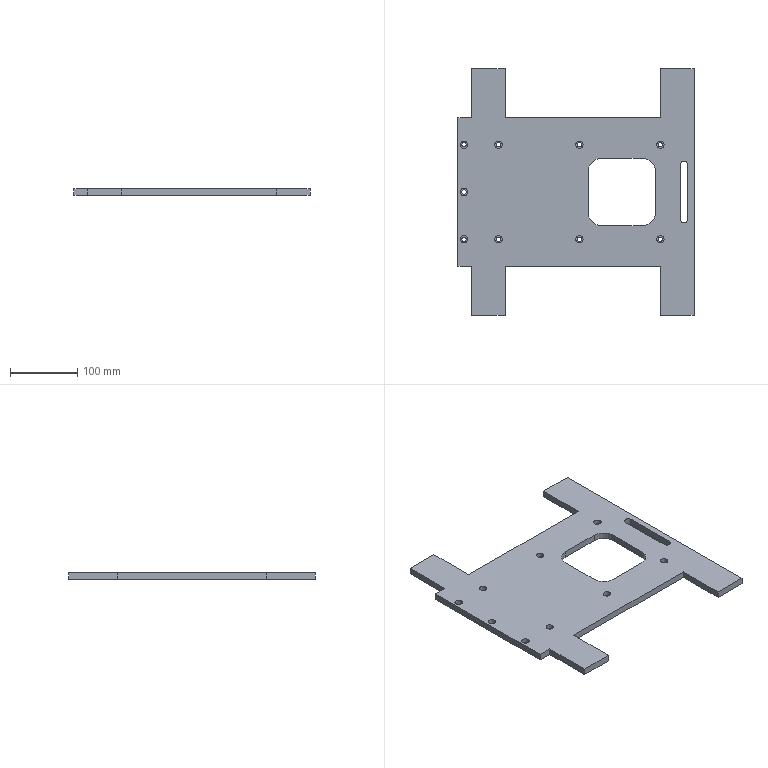Part | SolidWorks | features ICE 3, 3DProfileFeature 1, Extrusion 1, HoleWzd 1, LPattern 1 | 1 solid | 75 faces | box 350 x 366 x 10 mm | volume 802882 mm3 | cylinder 42 | plane 33 | commonest cylinder face diameters 11 x20 6.6 x18 40 x4